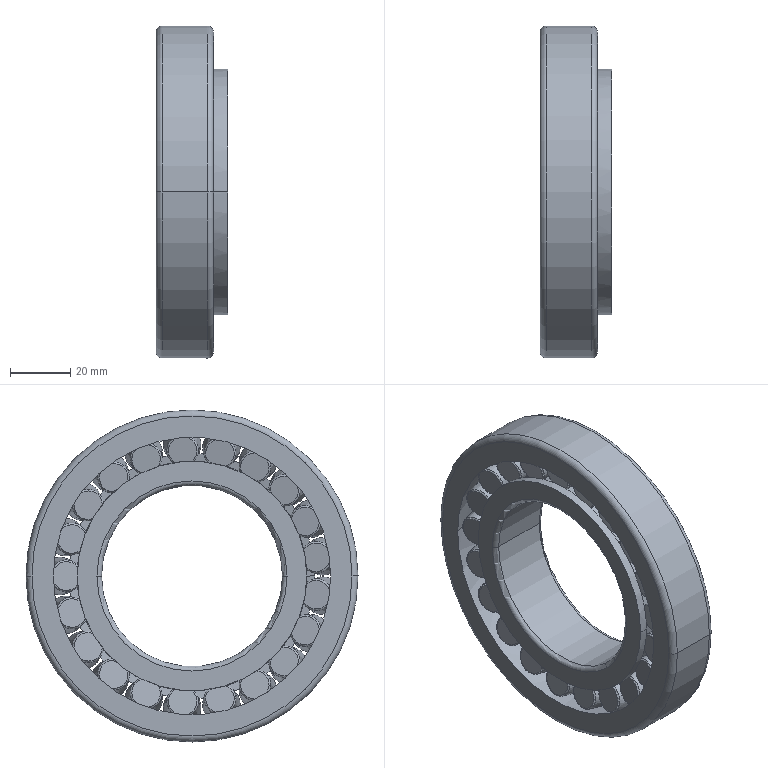Part | SolidWorks | features Revolution 3, CirPattern 1 | 1 solid | 196 faces | box 23.75 x 110 x 110 mm | volume 105381 mm3 | torus 92 | cone 50 | plane 46 | cylinder 8 | commonest cylinder face diameters 60 x2 76.07 x2 81.259 x2 110 x2